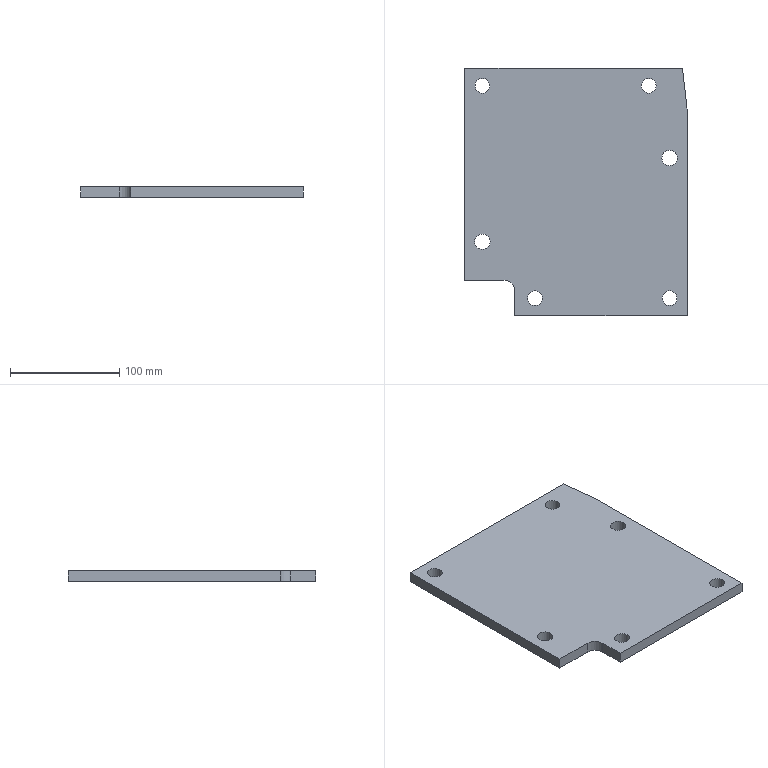Part | NX | features 6 2 | 1 solid | 16 faces | box 203 x 226 x 10 mm | volume 434534 mm3 | plane 9 | cylinder 7 | commonest cylinder face diameters 13.5 x4 14.001 x2 20 x1
STEP:
#1=CARTESIAN_POINT('',(210.63,11.939,91.));
#2=VERTEX_POINT('',#1);
#3=CARTESIAN_POINT('',(210.63,200.753,91.));
#4=VERTEX_POINT('',#3);
#5=CARTESIAN_POINT('',(210.63,119.939,91.));
#6=DIRECTION('',(0.,1.,0.));
#7=VECTOR('',#6,1000.);
#8=LINE('',#5,#7);
#9=EDGE_CURVE('',#2,#4,#8,.T.);
#10=ORIENTED_EDGE('',*,*,#9,.T.);
#11=CARTESIAN_POINT('',(210.63,200.753,101.));
#12=VERTEX_POINT('',#11);
#13=CARTESIAN_POINT('',(210.63,200.753,91.));
#14=DIRECTION('',(0.,0.,1.));
#15=VECTOR('',#14,1000.);
#16=LINE('',#13,#15);
#17=EDGE_CURVE('',#4,#12,#16,.T.);
#18=ORIENTED_EDGE('',*,*,#17,.T.);
#19=CARTESIAN_POINT('',(210.63,11.939,101.));
#20=VERTEX_POINT('',#19);
#21=CARTESIAN_POINT('',(210.63,119.939,101.));
#22=DIRECTION('',(0.,-1.,0.));
#23=VECTOR('',#22,1000.);
#24=LINE('',#21,#23);
#25=EDGE_CURVE('',#12,#20,#24,.T.);
#26=ORIENTED_EDGE('',*,*,#25,.T.);
#27=CARTESIAN_POINT('',(210.63,11.939,91.));
#28=DIRECTION('',(0.,0.,1.));
#29=VECTOR('',#28,1000.);
#30=LINE('',#27,#29);
#31=EDGE_CURVE('',#2,#20,#30,.T.);
#32=ORIENTED_EDGE('',*,*,#31,.F.);
#33=EDGE_LOOP('',(#10,#18,#26,#32));
#34=FACE_BOUND('',#33,.T.);
#35=CARTESIAN_POINT('',(210.63,119.939,91.));
#36=DIRECTION('',(1.,0.,0.));
#37=DIRECTION('',(0.,0.,1.));
#38=AXIS2_PLACEMENT_3D('',#35,#36,#37);
#39=PLANE('',#38);
#40=ADVANCED_FACE('',(#34),#39,.T.);
#41=CARTESIAN_POINT('',(7.63,237.939,101.));
#42=VERTEX_POINT('',#41);
#43=CARTESIAN_POINT('',(206.42,237.939,101.));
#44=VERTEX_POINT('',#43);
#45=CARTESIAN_POINT('',(102.63,237.939,101.));
#46=DIRECTION('',(1.,0.,0.));
#47=VECTOR('',#46,1000.);
#48=LINE('',#45,#47);
#49=EDGE_CURVE('',#42,#44,#48,.T.);
#50=ORIENTED_EDGE('',*,*,#49,.T.);
#51=CARTESIAN_POINT('',(206.42,237.939,91.));
#52=VERTEX_POINT('',#51);
#53=CARTESIAN_POINT('',(206.42,237.939,91.));
#54=DIRECTION('',(0.,0.,-1.));
#55=VECTOR('',#54,1000.);
#56=LINE('',#53,#55);
#57=EDGE_CURVE('',#44,#52,#56,.T.);
#58=ORIENTED_EDGE('',*,*,#57,.T.);
#59=CARTESIAN_POINT('',(7.63,237.939,91.));
#60=VERTEX_POINT('',#59);
#61=CARTESIAN_POINT('',(102.63,237.939,91.));
#62=DIRECTION('',(-1.,0.,0.));
#63=VECTOR('',#62,1000.);
#64=LINE('',#61,#63);
#65=EDGE_CURVE('',#52,#60,#64,.T.);
#66=ORIENTED_EDGE('',*,*,#65,.T.);
#67=CARTESIAN_POINT('',(7.63,237.939,91.));
#68=DIRECTION('',(0.,0.,1.));
#69=VECTOR('',#68,1000.);
#70=LINE('',#67,#69);
#71=EDGE_CURVE('',#60,#42,#70,.T.);
#72=ORIENTED_EDGE('',*,*,#71,.T.);
#73=EDGE_LOOP('',(#50,#58,#66,#72));
#74=FACE_BOUND('',#73,.T.);
#75=CARTESIAN_POINT('',(102.63,237.939,91.));
#76=DIRECTION('',(0.,1.,0.));
#77=DIRECTION('',(0.,0.,-1.));
#78=AXIS2_PLACEMENT_3D('',#75,#76,#77);
#79=PLANE('',#78);
#80=ADVANCED_FACE('',(#74),#79,.T.);
#81=CARTESIAN_POINT('',(201.63,155.939,101.));
#82=VERTEX_POINT('',#81);
#83=CARTESIAN_POINT('',(194.63,155.939,101.));
#84=DIRECTION('',(0.,0.,-1.));
#85=DIRECTION('',(1.,0.,0.));
#86=AXIS2_PLACEMENT_3D('',#83,#84,#85);
#87=CIRCLE('',#86,7.);
#88=EDGE_CURVE('',#82,#82,#87,.T.);
#89=ORIENTED_EDGE('',*,*,#88,.T.);
#90=EDGE_LOOP('',(#89));
#91=FACE_BOUND('',#90,.T.);
#92=CARTESIAN_POINT('',(30.38,221.939,101.));
#93=VERTEX_POINT('',#92);
#94=CARTESIAN_POINT('',(23.63,221.939,101.));
#95=DIRECTION('',(0.,0.,-1.));
#96=DIRECTION('',(1.,0.,0.));
#97=AXIS2_PLACEMENT_3D('',#94,#95,#96);
#98=CIRCLE('',#97,6.75);
#99=EDGE_CURVE('',#93,#93,#98,.T.);
#100=ORIENTED_EDGE('',*,*,#99,.T.);
#101=EDGE_LOOP('',(#100));
#102=FACE_BOUND('',#101,.T.);
#103=CARTESIAN_POINT('',(182.38,221.939,101.));
#104=VERTEX_POINT('',#103);
#105=CARTESIAN_POINT('',(175.63,221.939,101.));
#106=DIRECTION('',(0.,0.,-1.));
#107=DIRECTION('',(1.,0.,0.));
#108=AXIS2_PLACEMENT_3D('',#105,#106,#107);
#109=CIRCLE('',#108,6.75);
#110=EDGE_CURVE('',#104,#104,#109,.T.);
#111=ORIENTED_EDGE('',*,*,#110,.T.);
#112=EDGE_LOOP('',(#111));
#113=FACE_BOUND('',#112,.T.);
#114=CARTESIAN_POINT('',(201.38,27.939,101.));
#115=VERTEX_POINT('',#114);
#116=CARTESIAN_POINT('',(194.63,27.939,101.));
#117=DIRECTION('',(0.,0.,-1.));
#118=DIRECTION('',(1.,0.,0.));
#119=AXIS2_PLACEMENT_3D('',#116,#117,#118);
#120=CIRCLE('',#119,6.75);
#121=EDGE_CURVE('',#115,#115,#120,.T.);
#122=ORIENTED_EDGE('',*,*,#121,.T.);
#123=EDGE_LOOP('',(#122));
#124=FACE_BOUND('',#123,.T.);
#125=CARTESIAN_POINT('',(30.63,79.439,101.));
#126=VERTEX_POINT('',#125);
#127=CARTESIAN_POINT('',(23.63,79.439,101.));
#128=DIRECTION('',(0.,0.,-1.));
#129=DIRECTION('',(1.,0.,0.));
#130=AXIS2_PLACEMENT_3D('',#127,#128,#129);
#131=CIRCLE('',#130,7.);
#132=EDGE_CURVE('',#126,#126,#131,.T.);
#133=ORIENTED_EDGE('',*,*,#132,.T.);
#134=EDGE_LOOP('',(#133));
#135=FACE_BOUND('',#134,.T.);
#136=CARTESIAN_POINT('',(78.38,27.939,101.));
#137=VERTEX_POINT('',#136);
#138=CARTESIAN_POINT('',(71.63,27.939,101.));
#139=DIRECTION('',(0.,0.,1.));
#140=DIRECTION('',(1.,0.,0.));
#141=AXIS2_PLACEMENT_3D('',#138,#139,#140);
#142=CIRCLE('',#141,6.75);
#143=EDGE_CURVE('',#137,#137,#142,.T.);
#144=ORIENTED_EDGE('',*,*,#143,.F.);
#145=EDGE_LOOP('',(#144));
#146=FACE_BOUND('',#145,.T.);
#147=ORIENTED_EDGE('',*,*,#25,.F.);
#148=CARTESIAN_POINT('',(218.296,133.032,101.));
#149=DIRECTION('',(-0.1125,0.9937,0.));
#150=VECTOR('',#149,1000.);
#151=LINE('',#148,#150);
#152=EDGE_CURVE('',#12,#44,#151,.T.);
#153=ORIENTED_EDGE('',*,*,#152,.T.);
#154=ORIENTED_EDGE('',*,*,#49,.F.);
#155=CARTESIAN_POINT('',(7.63,44.5,101.));
#156=VERTEX_POINT('',#155);
#157=CARTESIAN_POINT('',(7.63,119.939,101.));
#158=DIRECTION('',(0.,1.,0.));
#159=VECTOR('',#158,1000.);
#160=LINE('',#157,#159);
#161=EDGE_CURVE('',#156,#42,#160,.T.);
#162=ORIENTED_EDGE('',*,*,#161,.F.);
#163=CARTESIAN_POINT('',(43.306,44.5,101.));
#164=VERTEX_POINT('',#163);
#165=CARTESIAN_POINT('',(102.63,44.5,101.));
#166=DIRECTION('',(-1.,0.,0.));
#167=VECTOR('',#166,1000.);
#168=LINE('',#165,#167);
#169=EDGE_CURVE('',#164,#156,#168,.T.);
#170=ORIENTED_EDGE('',*,*,#169,.F.);
#171=CARTESIAN_POINT('',(53.306,34.5,101.));
#172=VERTEX_POINT('',#171);
#173=CARTESIAN_POINT('',(43.306,34.5,101.));
#174=DIRECTION('',(0.,0.,-1.));
#175=DIRECTION('',(1.,0.,0.));
#176=AXIS2_PLACEMENT_3D('',#173,#174,#175);
#177=CIRCLE('',#176,10.);
#178=EDGE_CURVE('',#164,#172,#177,.T.);
#179=ORIENTED_EDGE('',*,*,#178,.T.);
#180=CARTESIAN_POINT('',(53.306,11.939,101.));
#181=VERTEX_POINT('',#180);
#182=CARTESIAN_POINT('',(53.306,-30.,101.));
#183=DIRECTION('',(0.,-1.,0.));
#184=VECTOR('',#183,1000.);
#185=LINE('',#182,#184);
#186=EDGE_CURVE('',#172,#181,#185,.T.);
#187=ORIENTED_EDGE('',*,*,#186,.T.);
#188=CARTESIAN_POINT('',(102.63,11.939,101.));
#189=DIRECTION('',(-1.,0.,0.));
#190=VECTOR('',#189,1000.);
#191=LINE('',#188,#190);
#192=EDGE_CURVE('',#20,#181,#191,.T.);
#193=ORIENTED_EDGE('',*,*,#192,.F.);
#194=EDGE_LOOP('',(#147,#153,#154,#162,#170,#179,#187,#193));
#195=FACE_BOUND('',#194,.T.);
#196=CARTESIAN_POINT('',(102.63,119.939,101.));
#197=DIRECTION('',(0.,0.,1.));
#198=DIRECTION('',(-1.,0.,0.));
#199=AXIS2_PLACEMENT_3D('',#196,#197,#198);
#200=PLANE('',#199);
#201=ADVANCED_FACE('',(#91,#102,#113,#124,#135,#146,#195),#200,.T.);
#202=CARTESIAN_POINT('',(201.63,155.939,91.));
#203=VERTEX_POINT('',#202);
#204=CARTESIAN_POINT('',(194.63,155.939,91.));
#205=DIRECTION('',(0.,0.,1.));
#206=DIRECTION('',(1.,0.,0.));
#207=AXIS2_PLACEMENT_3D('',#204,#205,#206);
#208=CIRCLE('',#207,7.);
#209=EDGE_CURVE('',#203,#203,#208,.T.);
#210=ORIENTED_EDGE('',*,*,#209,.T.);
#211=EDGE_LOOP('',(#210));
#212=FACE_BOUND('',#211,.T.);
#213=CARTESIAN_POINT('',(30.38,221.939,91.));
#214=VERTEX_POINT('',#213);
#215=CARTESIAN_POINT('',(23.63,221.939,91.));
#216=DIRECTION('',(0.,0.,1.));
#217=DIRECTION('',(1.,0.,0.));
#218=AXIS2_PLACEMENT_3D('',#215,#216,#217);
#219=CIRCLE('',#218,6.75);
#220=EDGE_CURVE('',#214,#214,#219,.T.);
#221=ORIENTED_EDGE('',*,*,#220,.T.);
#222=EDGE_LOOP('',(#221));
#223=FACE_BOUND('',#222,.T.);
#224=CARTESIAN_POINT('',(182.38,221.939,91.));
#225=VERTEX_POINT('',#224);
#226=CARTESIAN_POINT('',(175.63,221.939,91.));
#227=DIRECTION('',(0.,0.,1.));
#228=DIRECTION('',(1.,0.,0.));
#229=AXIS2_PLACEMENT_3D('',#226,#227,#228);
#230=CIRCLE('',#229,6.75);
#231=EDGE_CURVE('',#225,#225,#230,.T.);
#232=ORIENTED_EDGE('',*,*,#231,.T.);
#233=EDGE_LOOP('',(#232));
#234=FACE_BOUND('',#233,.T.);
#235=CARTESIAN_POINT('',(201.38,27.939,91.));
#236=VERTEX_POINT('',#235);
#237=CARTESIAN_POINT('',(194.63,27.939,91.));
#238=DIRECTION('',(0.,0.,1.));
#239=DIRECTION('',(1.,0.,0.));
#240=AXIS2_PLACEMENT_3D('',#237,#238,#239);
#241=CIRCLE('',#240,6.75);
#242=EDGE_CURVE('',#236,#236,#241,.T.);
#243=ORIENTED_EDGE('',*,*,#242,.T.);
#244=EDGE_LOOP('',(#243));
#245=FACE_BOUND('',#244,.T.);
#246=CARTESIAN_POINT('',(30.63,79.439,91.));
#247=VERTEX_POINT('',#246);
#248=CARTESIAN_POINT('',(23.63,79.439,91.));
#249=DIRECTION('',(0.,0.,1.));
#250=DIRECTION('',(1.,0.,0.));
#251=AXIS2_PLACEMENT_3D('',#248,#249,#250);
#252=CIRCLE('',#251,7.);
#253=EDGE_CURVE('',#247,#247,#252,.T.);
#254=ORIENTED_EDGE('',*,*,#253,.T.);
#255=EDGE_LOOP('',(#254));
#256=FACE_BOUND('',#255,.T.);
#257=CARTESIAN_POINT('',(64.88,27.939,91.));
#258=VERTEX_POINT('',#257);
#259=CARTESIAN_POINT('',(71.63,27.939,91.));
#260=DIRECTION('',(0.,0.,-1.));
#261=DIRECTION('',(-1.,0.,0.));
#262=AXIS2_PLACEMENT_3D('',#259,#260,#261);
#263=CIRCLE('',#262,6.75);
#264=EDGE_CURVE('',#258,#258,#263,.T.);
#265=ORIENTED_EDGE('',*,*,#264,.F.);
#266=EDGE_LOOP('',(#265));
#267=FACE_BOUND('',#266,.T.);
#268=ORIENTED_EDGE('',*,*,#65,.F.);
#269=CARTESIAN_POINT('',(218.296,133.032,91.));
#270=DIRECTION('',(0.1125,-0.9937,0.));
#271=VECTOR('',#270,1000.);
#272=LINE('',#269,#271);
#273=EDGE_CURVE('',#52,#4,#272,.T.);
#274=ORIENTED_EDGE('',*,*,#273,.T.);
#275=ORIENTED_EDGE('',*,*,#9,.F.);
#276=CARTESIAN_POINT('',(53.306,11.939,91.));
#277=VERTEX_POINT('',#276);
#278=CARTESIAN_POINT('',(102.63,11.939,91.));
#279=DIRECTION('',(1.,0.,0.));
#280=VECTOR('',#279,1000.);
#281=LINE('',#278,#280);
#282=EDGE_CURVE('',#277,#2,#281,.T.);
#283=ORIENTED_EDGE('',*,*,#282,.F.);
#284=CARTESIAN_POINT('',(53.306,34.5,91.));
#285=VERTEX_POINT('',#284);
#286=CARTESIAN_POINT('',(53.306,119.939,91.));
#287=DIRECTION('',(0.,-1.,0.));
#288=VECTOR('',#287,1000.);
#289=LINE('',#286,#288);
#290=EDGE_CURVE('',#285,#277,#289,.T.);
#291=ORIENTED_EDGE('',*,*,#290,.F.);
#292=CARTESIAN_POINT('',(43.306,44.5,91.));
#293=VERTEX_POINT('',#292);
#294=CARTESIAN_POINT('',(43.306,34.5,91.));
#295=DIRECTION('',(0.,0.,1.));
#296=DIRECTION('',(-1.,0.,0.));
#297=AXIS2_PLACEMENT_3D('',#294,#295,#296);
#298=CIRCLE('',#297,10.);
#299=EDGE_CURVE('',#285,#293,#298,.T.);
#300=ORIENTED_EDGE('',*,*,#299,.T.);
#301=CARTESIAN_POINT('',(7.63,44.5,91.));
#302=VERTEX_POINT('',#301);
#303=CARTESIAN_POINT('',(63.806,44.5,91.));
#304=DIRECTION('',(-1.,0.,0.));
#305=VECTOR('',#304,1000.);
#306=LINE('',#303,#305);
#307=EDGE_CURVE('',#293,#302,#306,.T.);
#308=ORIENTED_EDGE('',*,*,#307,.T.);
#309=CARTESIAN_POINT('',(7.63,119.939,91.));
#310=DIRECTION('',(0.,-1.,0.));
#311=VECTOR('',#310,1000.);
#312=LINE('',#309,#311);
#313=EDGE_CURVE('',#60,#302,#312,.T.);
#314=ORIENTED_EDGE('',*,*,#313,.F.);
#315=EDGE_LOOP('',(#268,#274,#275,#283,#291,#300,#308,#314));
#316=FACE_BOUND('',#315,.T.);
#317=CARTESIAN_POINT('',(102.63,119.939,91.));
#318=DIRECTION('',(0.,0.,-1.));
#319=DIRECTION('',(1.,0.,0.));
#320=AXIS2_PLACEMENT_3D('',#317,#318,#319);
#321=PLANE('',#320);
#322=ADVANCED_FACE('',(#212,#223,#234,#245,#256,#267,#316),#321,.T.);
#323=ORIENTED_EDGE('',*,*,#88,.F.);
#324=EDGE_LOOP('',(#323));
#325=FACE_BOUND('',#324,.T.);
#326=ORIENTED_EDGE('',*,*,#209,.F.);
#327=EDGE_LOOP('',(#326));
#328=FACE_BOUND('',#327,.T.);
#329=CARTESIAN_POINT('',(194.63,155.939,91.));
#330=DIRECTION('',(0.,0.,1.));
#331=DIRECTION('',(-1.,0.,0.));
#332=AXIS2_PLACEMENT_3D('',#329,#330,#331);
#333=CYLINDRICAL_SURFACE('',#332,7.);
#334=ADVANCED_FACE('',(#325,#328),#333,.F.);
#335=ORIENTED_EDGE('',*,*,#99,.F.);
#336=EDGE_LOOP('',(#335));
#337=FACE_BOUND('',#336,.T.);
#338=ORIENTED_EDGE('',*,*,#220,.F.);
#339=EDGE_LOOP('',(#338));
#340=FACE_BOUND('',#339,.T.);
#341=CARTESIAN_POINT('',(23.63,221.939,91.));
#342=DIRECTION('',(0.,0.,1.));
#343=DIRECTION('',(-1.,0.,0.));
#344=AXIS2_PLACEMENT_3D('',#341,#342,#343);
#345=CYLINDRICAL_SURFACE('',#344,6.75);
#346=ADVANCED_FACE('',(#337,#340),#345,.F.);
#347=ORIENTED_EDGE('',*,*,#110,.F.);
#348=EDGE_LOOP('',(#347));
#349=FACE_BOUND('',#348,.T.);
#350=ORIENTED_EDGE('',*,*,#231,.F.);
#351=EDGE_LOOP('',(#350));
#352=FACE_BOUND('',#351,.T.);
#353=CARTESIAN_POINT('',(175.63,221.939,91.));
#354=DIRECTION('',(0.,0.,1.));
#355=DIRECTION('',(-1.,0.,0.));
#356=AXIS2_PLACEMENT_3D('',#353,#354,#355);
#357=CYLINDRICAL_SURFACE('',#356,6.75);
#358=ADVANCED_FACE('',(#349,#352),#357,.F.);
#359=ORIENTED_EDGE('',*,*,#121,.F.);
#360=EDGE_LOOP('',(#359));
#361=FACE_BOUND('',#360,.T.);
#362=ORIENTED_EDGE('',*,*,#242,.F.);
#363=EDGE_LOOP('',(#362));
#364=FACE_BOUND('',#363,.T.);
#365=CARTESIAN_POINT('',(194.63,27.939,91.));
#366=DIRECTION('',(0.,0.,1.));
#367=DIRECTION('',(-1.,0.,0.));
#368=AXIS2_PLACEMENT_3D('',#365,#366,#367);
#369=CYLINDRICAL_SURFACE('',#368,6.75);
#370=ADVANCED_FACE('',(#361,#364),#369,.F.);
#371=ORIENTED_EDGE('',*,*,#132,.F.);
#372=EDGE_LOOP('',(#371));
#373=FACE_BOUND('',#372,.T.);
#374=ORIENTED_EDGE('',*,*,#253,.F.);
#375=EDGE_LOOP('',(#374));
#376=FACE_BOUND('',#375,.T.);
#377=CARTESIAN_POINT('',(23.63,79.439,91.));
#378=DIRECTION('',(0.,0.,1.));
#379=DIRECTION('',(-1.,0.,0.));
#380=AXIS2_PLACEMENT_3D('',#377,#378,#379);
#381=CYLINDRICAL_SURFACE('',#380,7.);
#382=ADVANCED_FACE('',(#373,#376),#381,.F.);
#383=CARTESIAN_POINT('',(7.63,44.5,-54.));
#384=DIRECTION('',(0.,0.,1.));
#385=VECTOR('',#384,1000.);
#386=LINE('',#383,#385);
#387=EDGE_CURVE('',#302,#156,#386,.T.);
#388=ORIENTED_EDGE('',*,*,#387,.T.);
#389=ORIENTED_EDGE('',*,*,#161,.T.);
#390=ORIENTED_EDGE('',*,*,#71,.F.);
#391=ORIENTED_EDGE('',*,*,#313,.T.);
#392=EDGE_LOOP('',(#388,#389,#390,#391));
#393=FACE_BOUND('',#392,.T.);
#394=CARTESIAN_POINT('',(7.63,119.939,91.));
#395=DIRECTION('',(-1.,0.,0.));
#396=DIRECTION('',(0.,0.,-1.));
#397=AXIS2_PLACEMENT_3D('',#394,#395,#396);
#398=PLANE('',#397);
#399=ADVANCED_FACE('',(#393),#398,.T.);
#400=CARTESIAN_POINT('',(53.306,11.939,91.));
#401=DIRECTION('',(0.,0.,1.));
#402=VECTOR('',#401,1000.);
#403=LINE('',#400,#402);
#404=EDGE_CURVE('',#277,#181,#403,.T.);
#405=ORIENTED_EDGE('',*,*,#404,.F.);
#406=ORIENTED_EDGE('',*,*,#282,.T.);
#407=ORIENTED_EDGE('',*,*,#31,.T.);
#408=ORIENTED_EDGE('',*,*,#192,.T.);
#409=EDGE_LOOP('',(#405,#406,#407,#408));
#410=FACE_BOUND('',#409,.T.);
#411=CARTESIAN_POINT('',(102.63,11.939,91.));
#412=DIRECTION('',(0.,-1.,0.));
#413=DIRECTION('',(0.,0.,1.));
#414=AXIS2_PLACEMENT_3D('',#411,#412,#413);
#415=PLANE('',#414);
#416=ADVANCED_FACE('',(#410),#415,.T.);
#417=ORIENTED_EDGE('',*,*,#186,.F.);
#418=CARTESIAN_POINT('',(53.306,34.5,91.));
#419=DIRECTION('',(0.,0.,-1.));
#420=VECTOR('',#419,1000.);
#421=LINE('',#418,#420);
#422=EDGE_CURVE('',#172,#285,#421,.T.);
#423=ORIENTED_EDGE('',*,*,#422,.T.);
#424=ORIENTED_EDGE('',*,*,#290,.T.);
#425=ORIENTED_EDGE('',*,*,#404,.T.);
#426=EDGE_LOOP('',(#417,#423,#424,#425));
#427=FACE_BOUND('',#426,.T.);
#428=CARTESIAN_POINT('',(53.306,-30.,-54.));
#429=DIRECTION('',(1.,0.,0.));
#430=DIRECTION('',(0.,0.,1.));
#431=AXIS2_PLACEMENT_3D('',#428,#429,#430);
#432=PLANE('',#431);
#433=ADVANCED_FACE('',(#427),#432,.F.);
#434=ORIENTED_EDGE('',*,*,#178,.F.);
#435=CARTESIAN_POINT('',(43.306,44.5,106.));
#436=DIRECTION('',(0.,0.,1.));
#437=VECTOR('',#436,1000.);
#438=LINE('',#435,#437);
#439=EDGE_CURVE('',#293,#164,#438,.T.);
#440=ORIENTED_EDGE('',*,*,#439,.F.);
#441=ORIENTED_EDGE('',*,*,#299,.F.);
#442=ORIENTED_EDGE('',*,*,#422,.F.);
#443=EDGE_LOOP('',(#434,#440,#441,#442));
#444=FACE_BOUND('',#443,.T.);
#445=CARTESIAN_POINT('',(43.306,34.5,-54.));
#446=DIRECTION('',(0.,0.,1.));
#447=DIRECTION('',(-1.,0.,0.));
#448=AXIS2_PLACEMENT_3D('',#445,#446,#447);
#449=CYLINDRICAL_SURFACE('',#448,10.);
#450=ADVANCED_FACE('',(#444),#449,.F.);
#451=ORIENTED_EDGE('',*,*,#307,.F.);
#452=ORIENTED_EDGE('',*,*,#439,.T.);
#453=ORIENTED_EDGE('',*,*,#169,.T.);
#454=ORIENTED_EDGE('',*,*,#387,.F.);
#455=EDGE_LOOP('',(#451,#452,#453,#454));
#456=FACE_BOUND('',#455,.T.);
#457=CARTESIAN_POINT('',(63.806,44.5,-54.));
#458=DIRECTION('',(0.,1.,0.));
#459=DIRECTION('',(0.,0.,-1.));
#460=AXIS2_PLACEMENT_3D('',#457,#458,#459);
#461=PLANE('',#460);
#462=ADVANCED_FACE('',(#456),#461,.F.);
#463=ORIENTED_EDGE('',*,*,#143,.T.);
#464=EDGE_LOOP('',(#463));
#465=FACE_BOUND('',#464,.T.);
#466=ORIENTED_EDGE('',*,*,#264,.T.);
#467=EDGE_LOOP('',(#466));
#468=FACE_BOUND('',#467,.T.);
#469=CARTESIAN_POINT('',(71.63,27.939,91.));
#470=DIRECTION('',(0.,0.,1.));
#471=DIRECTION('',(-1.,0.,0.));
#472=AXIS2_PLACEMENT_3D('',#469,#470,#471);
#473=CYLINDRICAL_SURFACE('',#472,6.75);
#474=ADVANCED_FACE('',(#465,#468),#473,.F.);
#475=ORIENTED_EDGE('',*,*,#152,.F.);
#476=ORIENTED_EDGE('',*,*,#17,.F.);
#477=ORIENTED_EDGE('',*,*,#273,.F.);
#478=ORIENTED_EDGE('',*,*,#57,.F.);
#479=EDGE_LOOP('',(#475,#476,#477,#478));
#480=FACE_BOUND('',#479,.T.);
#481=CARTESIAN_POINT('',(203.681,262.136,70.5));
#482=DIRECTION('',(0.9937,0.1125,0.));
#483=DIRECTION('',(0.1125,-0.9937,0.));
#484=AXIS2_PLACEMENT_3D('',#481,#482,#483);
#485=PLANE('',#484);
#486=ADVANCED_FACE('',(#480),#485,.T.);
#487=CLOSED_SHELL('',(#40,#80,#201,#322,#334,#346,#358,#370,#382,#399,#416,#433,#450,#462,#474,#486));
#488=MANIFOLD_SOLID_BREP('',#487);
#489=(LENGTH_UNIT()NAMED_UNIT(*)SI_UNIT(.MILLI.,.METRE.));
#490=UNCERTAINTY_MEASURE_WITH_UNIT(LENGTH_MEASURE(0.00001),#489,'','');
#491=(NAMED_UNIT(*)PLANE_ANGLE_UNIT()SI_UNIT($,.RADIAN.));
#492=(NAMED_UNIT(*)SI_UNIT($,.STERADIAN.)SOLID_ANGLE_UNIT());
#493=(GEOMETRIC_REPRESENTATION_CONTEXT(3)GLOBAL_UNCERTAINTY_ASSIGNED_CONTEXT((#490))GLOBAL_UNIT_ASSIGNED_CONTEXT((#489,#491,#492))REPRESENTATION_CONTEXT('',''));
#494=ADVANCED_BREP_SHAPE_REPRESENTATION('',(#488),#493);